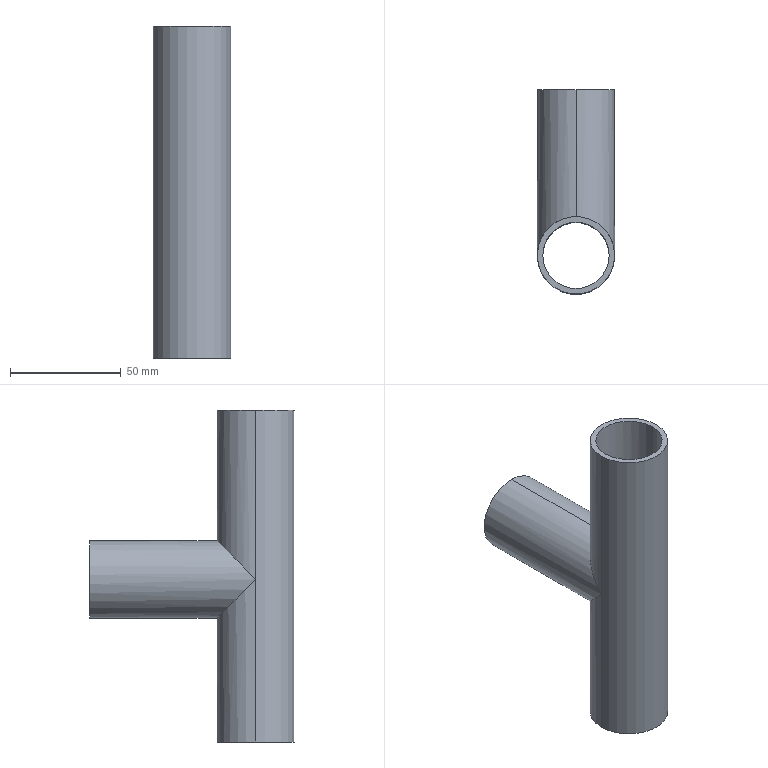Part | SolidWorks | features BaseBody 1 | 1 solid | 13 faces | box 35 x 92.5 x 150 mm | volume 52141 mm3 | cylinder 10 | plane 3 | commonest cylinder face diameters 30 x5 35 x5
STEP:
#1=CARTESIAN_POINT('',(-17.5,0.,150.));
#2=VERTEX_POINT('',#1);
#3=CARTESIAN_POINT('',(17.5,0.,150.));
#4=VERTEX_POINT('',#3);
#5=CARTESIAN_POINT('',(0.,0.,150.));
#6=DIRECTION('',(0.,0.,-1.));
#7=DIRECTION('',(-1.,0.,0.));
#8=AXIS2_PLACEMENT_3D('',#5,#6,#7);
#9=CIRCLE('',#8,17.5);
#10=EDGE_CURVE('',#2,#4,#9,.T.);
#11=ORIENTED_EDGE('',*,*,#10,.T.);
#12=CARTESIAN_POINT('',(17.5,0.,73.465));
#13=VERTEX_POINT('',#12);
#14=CARTESIAN_POINT('',(17.5,0.,150.));
#15=DIRECTION('',(0.,0.,-1.));
#16=VECTOR('',#15,1000.);
#17=LINE('',#14,#16);
#18=EDGE_CURVE('',#4,#13,#17,.T.);
#19=ORIENTED_EDGE('',*,*,#18,.T.);
#20=CARTESIAN_POINT('',(0.,17.5,90.965));
#21=VERTEX_POINT('',#20);
#22=CARTESIAN_POINT('',(17.5,0.,73.465));
#23=CARTESIAN_POINT('',(17.5,10.251,83.716));
#24=CARTESIAN_POINT('',(10.251,17.5,90.965));
#25=CARTESIAN_POINT('',(0.,17.5,90.965));
#26=(BOUNDED_CURVE()B_SPLINE_CURVE(3,(#22,#23,#24,#25),.UNSPECIFIED.,.F.,.T.)B_SPLINE_CURVE_WITH_KNOTS((4,4),(1.571,3.142),.UNSPECIFIED.)CURVE()GEOMETRIC_REPRESENTATION_ITEM()RATIONAL_B_SPLINE_CURVE((1.,0.8047,0.8047,1.))REPRESENTATION_ITEM(''));
#27=EDGE_CURVE('',#13,#21,#26,.T.);
#28=ORIENTED_EDGE('',*,*,#27,.T.);
#29=CARTESIAN_POINT('',(-17.5,0.,73.465));
#30=VERTEX_POINT('',#29);
#31=CARTESIAN_POINT('',(0.,17.5,90.965));
#32=CARTESIAN_POINT('',(-10.251,17.5,90.965));
#33=CARTESIAN_POINT('',(-17.5,10.251,83.716));
#34=CARTESIAN_POINT('',(-17.5,0.,73.465));
#35=(BOUNDED_CURVE()B_SPLINE_CURVE(3,(#31,#32,#33,#34),.UNSPECIFIED.,.F.,.F.)B_SPLINE_CURVE_WITH_KNOTS((4,4),(3.142,4.712),.UNSPECIFIED.)CURVE()GEOMETRIC_REPRESENTATION_ITEM()RATIONAL_B_SPLINE_CURVE((1.,0.8047,0.8047,1.))REPRESENTATION_ITEM(''));
#36=EDGE_CURVE('',#21,#30,#35,.T.);
#37=ORIENTED_EDGE('',*,*,#36,.T.);
#38=CARTESIAN_POINT('',(-17.5,0.,150.));
#39=DIRECTION('',(0.,0.,-1.));
#40=VECTOR('',#39,1000.);
#41=LINE('',#38,#40);
#42=EDGE_CURVE('',#2,#30,#41,.T.);
#43=ORIENTED_EDGE('',*,*,#42,.F.);
#44=EDGE_LOOP('',(#11,#19,#28,#37,#43));
#45=FACE_OUTER_BOUND('',#44,.T.);
#46=CARTESIAN_POINT('',(0.,0.,150.));
#47=DIRECTION('',(0.,0.,-1.));
#48=DIRECTION('',(-1.,0.,0.));
#49=AXIS2_PLACEMENT_3D('',#46,#47,#48);
#50=CYLINDRICAL_SURFACE('',#49,17.5);
#51=ADVANCED_FACE('',(#45),#50,.T.);
#52=CARTESIAN_POINT('',(0.,17.5,55.965));
#53=VERTEX_POINT('',#52);
#54=CARTESIAN_POINT('',(0.,17.5,55.965));
#55=CARTESIAN_POINT('',(10.251,17.5,55.965));
#56=CARTESIAN_POINT('',(17.5,10.251,63.213));
#57=CARTESIAN_POINT('',(17.5,0.,73.465));
#58=(BOUNDED_CURVE()B_SPLINE_CURVE(3,(#54,#55,#56,#57),.UNSPECIFIED.,.F.,.T.)B_SPLINE_CURVE_WITH_KNOTS((4,4),(3.142,4.712),.UNSPECIFIED.)CURVE()GEOMETRIC_REPRESENTATION_ITEM()RATIONAL_B_SPLINE_CURVE((1.,0.8047,0.8047,1.))REPRESENTATION_ITEM(''));
#59=EDGE_CURVE('',#53,#13,#58,.T.);
#60=ORIENTED_EDGE('',*,*,#59,.T.);
#61=CARTESIAN_POINT('',(17.5,0.,0.));
#62=VERTEX_POINT('',#61);
#63=CARTESIAN_POINT('',(17.5,0.,150.));
#64=DIRECTION('',(0.,0.,-1.));
#65=VECTOR('',#64,1000.);
#66=LINE('',#63,#65);
#67=EDGE_CURVE('',#13,#62,#66,.T.);
#68=ORIENTED_EDGE('',*,*,#67,.T.);
#69=CARTESIAN_POINT('',(-17.5,0.,0.));
#70=VERTEX_POINT('',#69);
#71=CARTESIAN_POINT('',(0.,0.,0.));
#72=DIRECTION('',(0.,0.,1.));
#73=DIRECTION('',(-1.,0.,0.));
#74=AXIS2_PLACEMENT_3D('',#71,#72,#73);
#75=CIRCLE('',#74,17.5);
#76=EDGE_CURVE('',#62,#70,#75,.T.);
#77=ORIENTED_EDGE('',*,*,#76,.T.);
#78=CARTESIAN_POINT('',(-17.5,0.,150.));
#79=DIRECTION('',(0.,0.,-1.));
#80=VECTOR('',#79,1000.);
#81=LINE('',#78,#80);
#82=EDGE_CURVE('',#30,#70,#81,.T.);
#83=ORIENTED_EDGE('',*,*,#82,.F.);
#84=CARTESIAN_POINT('',(-17.5,0.,73.465));
#85=CARTESIAN_POINT('',(-17.5,10.251,63.213));
#86=CARTESIAN_POINT('',(-10.251,17.5,55.965));
#87=CARTESIAN_POINT('',(0.,17.5,55.965));
#88=(BOUNDED_CURVE()B_SPLINE_CURVE(3,(#84,#85,#86,#87),.UNSPECIFIED.,.F.,.F.)B_SPLINE_CURVE_WITH_KNOTS((4,4),(1.571,3.142),.UNSPECIFIED.)CURVE()GEOMETRIC_REPRESENTATION_ITEM()RATIONAL_B_SPLINE_CURVE((1.,0.8047,0.8047,1.))REPRESENTATION_ITEM(''));
#89=EDGE_CURVE('',#30,#53,#88,.T.);
#90=ORIENTED_EDGE('',*,*,#89,.T.);
#91=EDGE_LOOP('',(#60,#68,#77,#83,#90));
#92=FACE_OUTER_BOUND('',#91,.T.);
#93=CARTESIAN_POINT('',(0.,0.,150.));
#94=DIRECTION('',(0.,0.,-1.));
#95=DIRECTION('',(-1.,0.,0.));
#96=AXIS2_PLACEMENT_3D('',#93,#94,#95);
#97=CYLINDRICAL_SURFACE('',#96,17.5);
#98=ADVANCED_FACE('',(#92),#97,.T.);
#99=CARTESIAN_POINT('',(0.,75.,55.965));
#100=VERTEX_POINT('',#99);
#101=CARTESIAN_POINT('',(0.,75.,90.965));
#102=VERTEX_POINT('',#101);
#103=CARTESIAN_POINT('',(0.,75.,73.465));
#104=DIRECTION('',(0.,-1.,0.));
#105=DIRECTION('',(0.,0.,-1.));
#106=AXIS2_PLACEMENT_3D('',#103,#104,#105);
#107=CIRCLE('',#106,17.5);
#108=EDGE_CURVE('',#100,#102,#107,.T.);
#109=ORIENTED_EDGE('',*,*,#108,.T.);
#110=CARTESIAN_POINT('',(0.,75.,90.965));
#111=DIRECTION('',(0.,-1.,0.));
#112=VECTOR('',#111,1000.);
#113=LINE('',#110,#112);
#114=EDGE_CURVE('',#102,#21,#113,.T.);
#115=ORIENTED_EDGE('',*,*,#114,.T.);
#116=ORIENTED_EDGE('',*,*,#27,.F.);
#117=ORIENTED_EDGE('',*,*,#59,.F.);
#118=CARTESIAN_POINT('',(0.,75.,55.965));
#119=DIRECTION('',(0.,-1.,0.));
#120=VECTOR('',#119,1000.);
#121=LINE('',#118,#120);
#122=EDGE_CURVE('',#100,#53,#121,.T.);
#123=ORIENTED_EDGE('',*,*,#122,.F.);
#124=EDGE_LOOP('',(#109,#115,#116,#117,#123));
#125=FACE_OUTER_BOUND('',#124,.T.);
#126=CARTESIAN_POINT('',(0.,75.,73.465));
#127=DIRECTION('',(0.,-1.,0.));
#128=DIRECTION('',(0.,0.,-1.));
#129=AXIS2_PLACEMENT_3D('',#126,#127,#128);
#130=CYLINDRICAL_SURFACE('',#129,17.5);
#131=ADVANCED_FACE('',(#125),#130,.T.);
#132=CARTESIAN_POINT('',(15.,0.,150.));
#133=VERTEX_POINT('',#132);
#134=CARTESIAN_POINT('',(-15.,0.,150.));
#135=VERTEX_POINT('',#134);
#136=CARTESIAN_POINT('',(0.,0.,150.));
#137=DIRECTION('',(0.,0.,-1.));
#138=DIRECTION('',(-1.,0.,0.));
#139=AXIS2_PLACEMENT_3D('',#136,#137,#138);
#140=CIRCLE('',#139,15.);
#141=EDGE_CURVE('',#133,#135,#140,.T.);
#142=ORIENTED_EDGE('',*,*,#141,.F.);
#143=CARTESIAN_POINT('',(15.,0.,73.465));
#144=VERTEX_POINT('',#143);
#145=CARTESIAN_POINT('',(15.,0.,150.));
#146=DIRECTION('',(0.,0.,-1.));
#147=VECTOR('',#146,1000.);
#148=LINE('',#145,#147);
#149=EDGE_CURVE('',#133,#144,#148,.T.);
#150=ORIENTED_EDGE('',*,*,#149,.T.);
#151=CARTESIAN_POINT('',(15.,0.,0.));
#152=VERTEX_POINT('',#151);
#153=CARTESIAN_POINT('',(15.,0.,150.));
#154=DIRECTION('',(0.,0.,-1.));
#155=VECTOR('',#154,1000.);
#156=LINE('',#153,#155);
#157=EDGE_CURVE('',#144,#152,#156,.T.);
#158=ORIENTED_EDGE('',*,*,#157,.T.);
#159=CARTESIAN_POINT('',(-15.,0.,0.));
#160=VERTEX_POINT('',#159);
#161=CARTESIAN_POINT('',(0.,0.,0.));
#162=DIRECTION('',(0.,0.,-1.));
#163=DIRECTION('',(-1.,0.,0.));
#164=AXIS2_PLACEMENT_3D('',#161,#162,#163);
#165=CIRCLE('',#164,15.);
#166=EDGE_CURVE('',#152,#160,#165,.T.);
#167=ORIENTED_EDGE('',*,*,#166,.T.);
#168=CARTESIAN_POINT('',(-15.,0.,73.465));
#169=VERTEX_POINT('',#168);
#170=CARTESIAN_POINT('',(-15.,0.,150.));
#171=DIRECTION('',(0.,0.,-1.));
#172=VECTOR('',#171,1000.);
#173=LINE('',#170,#172);
#174=EDGE_CURVE('',#169,#160,#173,.T.);
#175=ORIENTED_EDGE('',*,*,#174,.F.);
#176=CARTESIAN_POINT('',(-15.,0.,150.));
#177=DIRECTION('',(0.,0.,-1.));
#178=VECTOR('',#177,1000.);
#179=LINE('',#176,#178);
#180=EDGE_CURVE('',#135,#169,#179,.T.);
#181=ORIENTED_EDGE('',*,*,#180,.F.);
#182=EDGE_LOOP('',(#142,#150,#158,#167,#175,#181));
#183=FACE_OUTER_BOUND('',#182,.T.);
#184=CARTESIAN_POINT('',(0.,0.,150.));
#185=DIRECTION('',(0.,0.,-1.));
#186=DIRECTION('',(-1.,0.,0.));
#187=AXIS2_PLACEMENT_3D('',#184,#185,#186);
#188=CYLINDRICAL_SURFACE('',#187,15.);
#189=ADVANCED_FACE('',(#183),#188,.F.);
#190=ORIENTED_EDGE('',*,*,#149,.F.);
#191=CARTESIAN_POINT('',(0.,0.,150.));
#192=DIRECTION('',(0.,0.,-1.));
#193=DIRECTION('',(-1.,0.,0.));
#194=AXIS2_PLACEMENT_3D('',#191,#192,#193);
#195=CIRCLE('',#194,15.);
#196=EDGE_CURVE('',#135,#133,#195,.T.);
#197=ORIENTED_EDGE('',*,*,#196,.F.);
#198=ORIENTED_EDGE('',*,*,#180,.T.);
#199=CARTESIAN_POINT('',(0.,15.,88.465));
#200=VERTEX_POINT('',#199);
#201=CARTESIAN_POINT('',(0.,15.,88.465));
#202=CARTESIAN_POINT('',(-8.787,15.,88.465));
#203=CARTESIAN_POINT('',(-15.,8.787,82.251));
#204=CARTESIAN_POINT('',(-15.,0.,73.465));
#205=(BOUNDED_CURVE()B_SPLINE_CURVE(3,(#201,#202,#203,#204),.UNSPECIFIED.,.F.,.F.)B_SPLINE_CURVE_WITH_KNOTS((4,4),(0.,1.571),.UNSPECIFIED.)CURVE()GEOMETRIC_REPRESENTATION_ITEM()RATIONAL_B_SPLINE_CURVE((1.,0.8047,0.8047,1.))REPRESENTATION_ITEM(''));
#206=EDGE_CURVE('',#200,#169,#205,.T.);
#207=ORIENTED_EDGE('',*,*,#206,.F.);
#208=CARTESIAN_POINT('',(15.,0.,73.465));
#209=CARTESIAN_POINT('',(15.,8.787,82.251));
#210=CARTESIAN_POINT('',(8.787,15.,88.465));
#211=CARTESIAN_POINT('',(0.,15.,88.465));
#212=(BOUNDED_CURVE()B_SPLINE_CURVE(3,(#208,#209,#210,#211),.UNSPECIFIED.,.F.,.F.)B_SPLINE_CURVE_WITH_KNOTS((4,4),(4.712,6.283),.UNSPECIFIED.)CURVE()GEOMETRIC_REPRESENTATION_ITEM()RATIONAL_B_SPLINE_CURVE((1.,0.8047,0.8047,1.))REPRESENTATION_ITEM(''));
#213=EDGE_CURVE('',#144,#200,#212,.T.);
#214=ORIENTED_EDGE('',*,*,#213,.F.);
#215=EDGE_LOOP('',(#190,#197,#198,#207,#214));
#216=FACE_OUTER_BOUND('',#215,.T.);
#217=CARTESIAN_POINT('',(0.,0.,150.));
#218=DIRECTION('',(0.,0.,-1.));
#219=DIRECTION('',(-1.,0.,0.));
#220=AXIS2_PLACEMENT_3D('',#217,#218,#219);
#221=CYLINDRICAL_SURFACE('',#220,15.);
#222=ADVANCED_FACE('',(#216),#221,.F.);
#223=CARTESIAN_POINT('',(0.,15.,58.465));
#224=VERTEX_POINT('',#223);
#225=CARTESIAN_POINT('',(-15.,0.,73.465));
#226=CARTESIAN_POINT('',(-15.,8.787,64.678));
#227=CARTESIAN_POINT('',(-8.787,15.,58.465));
#228=CARTESIAN_POINT('',(0.,15.,58.465));
#229=(BOUNDED_CURVE()B_SPLINE_CURVE(3,(#225,#226,#227,#228),.UNSPECIFIED.,.F.,.F.)B_SPLINE_CURVE_WITH_KNOTS((4,4),(4.712,6.283),.UNSPECIFIED.)CURVE()GEOMETRIC_REPRESENTATION_ITEM()RATIONAL_B_SPLINE_CURVE((1.,0.8047,0.8047,1.))REPRESENTATION_ITEM(''));
#230=EDGE_CURVE('',#169,#224,#229,.T.);
#231=ORIENTED_EDGE('',*,*,#230,.T.);
#232=CARTESIAN_POINT('',(0.,75.,58.465));
#233=VERTEX_POINT('',#232);
#234=CARTESIAN_POINT('',(0.,0.,58.465));
#235=DIRECTION('',(0.,1.,0.));
#236=VECTOR('',#235,1000.);
#237=LINE('',#234,#236);
#238=EDGE_CURVE('',#224,#233,#237,.T.);
#239=ORIENTED_EDGE('',*,*,#238,.T.);
#240=CARTESIAN_POINT('',(0.,75.,88.465));
#241=VERTEX_POINT('',#240);
#242=CARTESIAN_POINT('',(0.,75.,73.465));
#243=DIRECTION('',(0.,-1.,0.));
#244=DIRECTION('',(0.,0.,1.));
#245=AXIS2_PLACEMENT_3D('',#242,#243,#244);
#246=CIRCLE('',#245,15.);
#247=EDGE_CURVE('',#241,#233,#246,.T.);
#248=ORIENTED_EDGE('',*,*,#247,.F.);
#249=CARTESIAN_POINT('',(0.,0.,88.465));
#250=DIRECTION('',(0.,1.,0.));
#251=VECTOR('',#250,1000.);
#252=LINE('',#249,#251);
#253=EDGE_CURVE('',#200,#241,#252,.T.);
#254=ORIENTED_EDGE('',*,*,#253,.F.);
#255=ORIENTED_EDGE('',*,*,#206,.T.);
#256=EDGE_LOOP('',(#231,#239,#248,#254,#255));
#257=FACE_OUTER_BOUND('',#256,.T.);
#258=CARTESIAN_POINT('',(0.,0.,73.465));
#259=DIRECTION('',(0.,1.,0.));
#260=DIRECTION('',(0.,0.,1.));
#261=AXIS2_PLACEMENT_3D('',#258,#259,#260);
#262=CYLINDRICAL_SURFACE('',#261,15.);
#263=ADVANCED_FACE('',(#257),#262,.F.);
#264=ORIENTED_EDGE('',*,*,#18,.F.);
#265=CARTESIAN_POINT('',(0.,0.,150.));
#266=DIRECTION('',(0.,0.,-1.));
#267=DIRECTION('',(-1.,0.,0.));
#268=AXIS2_PLACEMENT_3D('',#265,#266,#267);
#269=CIRCLE('',#268,17.5);
#270=EDGE_CURVE('',#4,#2,#269,.T.);
#271=ORIENTED_EDGE('',*,*,#270,.T.);
#272=ORIENTED_EDGE('',*,*,#42,.T.);
#273=ORIENTED_EDGE('',*,*,#82,.T.);
#274=CARTESIAN_POINT('',(0.,0.,0.));
#275=DIRECTION('',(0.,0.,1.));
#276=DIRECTION('',(-1.,0.,0.));
#277=AXIS2_PLACEMENT_3D('',#274,#275,#276);
#278=CIRCLE('',#277,17.5);
#279=EDGE_CURVE('',#70,#62,#278,.T.);
#280=ORIENTED_EDGE('',*,*,#279,.T.);
#281=ORIENTED_EDGE('',*,*,#67,.F.);
#282=EDGE_LOOP('',(#264,#271,#272,#273,#280,#281));
#283=FACE_OUTER_BOUND('',#282,.T.);
#284=CARTESIAN_POINT('',(0.,0.,150.));
#285=DIRECTION('',(0.,0.,-1.));
#286=DIRECTION('',(-1.,0.,0.));
#287=AXIS2_PLACEMENT_3D('',#284,#285,#286);
#288=CYLINDRICAL_SURFACE('',#287,17.5);
#289=ADVANCED_FACE('',(#283),#288,.T.);
#290=CARTESIAN_POINT('',(0.,0.,0.));
#291=DIRECTION('',(0.,0.,-1.));
#292=DIRECTION('',(-1.,0.,0.));
#293=AXIS2_PLACEMENT_3D('',#290,#291,#292);
#294=CIRCLE('',#293,15.);
#295=EDGE_CURVE('',#160,#152,#294,.T.);
#296=ORIENTED_EDGE('',*,*,#295,.F.);
#297=ORIENTED_EDGE('',*,*,#166,.F.);
#298=EDGE_LOOP('',(#296,#297));
#299=FACE_BOUND('',#298,.T.);
#300=ORIENTED_EDGE('',*,*,#279,.F.);
#301=ORIENTED_EDGE('',*,*,#76,.F.);
#302=EDGE_LOOP('',(#300,#301));
#303=FACE_OUTER_BOUND('',#302,.T.);
#304=CARTESIAN_POINT('',(0.,0.,0.));
#305=DIRECTION('',(0.,0.,1.));
#306=DIRECTION('',(1.,0.,0.));
#307=AXIS2_PLACEMENT_3D('',#304,#305,#306);
#308=PLANE('',#307);
#309=ADVANCED_FACE('',(#299,#303),#308,.F.);
#310=ORIENTED_EDGE('',*,*,#196,.T.);
#311=ORIENTED_EDGE('',*,*,#141,.T.);
#312=EDGE_LOOP('',(#310,#311));
#313=FACE_BOUND('',#312,.T.);
#314=ORIENTED_EDGE('',*,*,#10,.F.);
#315=ORIENTED_EDGE('',*,*,#270,.F.);
#316=EDGE_LOOP('',(#314,#315));
#317=FACE_OUTER_BOUND('',#316,.T.);
#318=CARTESIAN_POINT('',(0.,0.,150.));
#319=DIRECTION('',(0.,0.,1.));
#320=DIRECTION('',(1.,0.,0.));
#321=AXIS2_PLACEMENT_3D('',#318,#319,#320);
#322=PLANE('',#321);
#323=ADVANCED_FACE('',(#313,#317),#322,.T.);
#324=ORIENTED_EDGE('',*,*,#114,.F.);
#325=CARTESIAN_POINT('',(0.,75.,73.465));
#326=DIRECTION('',(0.,-1.,0.));
#327=DIRECTION('',(0.,0.,-1.));
#328=AXIS2_PLACEMENT_3D('',#325,#326,#327);
#329=CIRCLE('',#328,17.5);
#330=EDGE_CURVE('',#102,#100,#329,.T.);
#331=ORIENTED_EDGE('',*,*,#330,.T.);
#332=ORIENTED_EDGE('',*,*,#122,.T.);
#333=ORIENTED_EDGE('',*,*,#89,.F.);
#334=ORIENTED_EDGE('',*,*,#36,.F.);
#335=EDGE_LOOP('',(#324,#331,#332,#333,#334));
#336=FACE_OUTER_BOUND('',#335,.T.);
#337=CARTESIAN_POINT('',(0.,75.,73.465));
#338=DIRECTION('',(0.,-1.,0.));
#339=DIRECTION('',(0.,0.,-1.));
#340=AXIS2_PLACEMENT_3D('',#337,#338,#339);
#341=CYLINDRICAL_SURFACE('',#340,17.5);
#342=ADVANCED_FACE('',(#336),#341,.T.);
#343=ORIENTED_EDGE('',*,*,#157,.F.);
#344=CARTESIAN_POINT('',(0.,15.,58.465));
#345=CARTESIAN_POINT('',(8.787,15.,58.465));
#346=CARTESIAN_POINT('',(15.,8.787,64.678));
#347=CARTESIAN_POINT('',(15.,0.,73.465));
#348=(BOUNDED_CURVE()B_SPLINE_CURVE(3,(#344,#345,#346,#347),.UNSPECIFIED.,.F.,.F.)B_SPLINE_CURVE_WITH_KNOTS((4,4),(0.,1.571),.UNSPECIFIED.)CURVE()GEOMETRIC_REPRESENTATION_ITEM()RATIONAL_B_SPLINE_CURVE((1.,0.8047,0.8047,1.))REPRESENTATION_ITEM(''));
#349=EDGE_CURVE('',#224,#144,#348,.T.);
#350=ORIENTED_EDGE('',*,*,#349,.F.);
#351=ORIENTED_EDGE('',*,*,#230,.F.);
#352=ORIENTED_EDGE('',*,*,#174,.T.);
#353=ORIENTED_EDGE('',*,*,#295,.T.);
#354=EDGE_LOOP('',(#343,#350,#351,#352,#353));
#355=FACE_OUTER_BOUND('',#354,.T.);
#356=CARTESIAN_POINT('',(0.,0.,150.));
#357=DIRECTION('',(0.,0.,-1.));
#358=DIRECTION('',(-1.,0.,0.));
#359=AXIS2_PLACEMENT_3D('',#356,#357,#358);
#360=CYLINDRICAL_SURFACE('',#359,15.);
#361=ADVANCED_FACE('',(#355),#360,.F.);
#362=ORIENTED_EDGE('',*,*,#108,.F.);
#363=ORIENTED_EDGE('',*,*,#330,.F.);
#364=EDGE_LOOP('',(#362,#363));
#365=FACE_OUTER_BOUND('',#364,.T.);
#366=ORIENTED_EDGE('',*,*,#247,.T.);
#367=CARTESIAN_POINT('',(0.,75.,73.465));
#368=DIRECTION('',(0.,-1.,0.));
#369=DIRECTION('',(0.,0.,1.));
#370=AXIS2_PLACEMENT_3D('',#367,#368,#369);
#371=CIRCLE('',#370,15.);
#372=EDGE_CURVE('',#233,#241,#371,.T.);
#373=ORIENTED_EDGE('',*,*,#372,.T.);
#374=EDGE_LOOP('',(#366,#373));
#375=FACE_BOUND('',#374,.T.);
#376=CARTESIAN_POINT('',(0.,75.,73.465));
#377=DIRECTION('',(0.,1.,0.));
#378=DIRECTION('',(0.,0.,1.));
#379=AXIS2_PLACEMENT_3D('',#376,#377,#378);
#380=PLANE('',#379);
#381=ADVANCED_FACE('',(#365,#375),#380,.T.);
#382=ORIENTED_EDGE('',*,*,#238,.F.);
#383=ORIENTED_EDGE('',*,*,#349,.T.);
#384=ORIENTED_EDGE('',*,*,#213,.T.);
#385=ORIENTED_EDGE('',*,*,#253,.T.);
#386=ORIENTED_EDGE('',*,*,#372,.F.);
#387=EDGE_LOOP('',(#382,#383,#384,#385,#386));
#388=FACE_OUTER_BOUND('',#387,.T.);
#389=CARTESIAN_POINT('',(0.,0.,73.465));
#390=DIRECTION('',(0.,1.,0.));
#391=DIRECTION('',(0.,0.,1.));
#392=AXIS2_PLACEMENT_3D('',#389,#390,#391);
#393=CYLINDRICAL_SURFACE('',#392,15.);
#394=ADVANCED_FACE('',(#388),#393,.F.);
#395=CLOSED_SHELL('',(#51,#98,#131,#189,#222,#263,#289,#309,#323,#342,#361,#381,#394));
#396=MANIFOLD_SOLID_BREP('',#395);
#397=CARTESIAN_POINT('',(0.,0.,0.));
#398=DIRECTION('',(0.,0.,1.));
#399=DIRECTION('',(1.,0.,0.));
#400=AXIS2_PLACEMENT_3D('',#397,#398,#399);
#401=(LENGTH_UNIT()NAMED_UNIT(*)SI_UNIT(.MILLI.,.METRE.));
#402=UNCERTAINTY_MEASURE_WITH_UNIT(LENGTH_MEASURE(0.00001),#401,'','');
#403=(NAMED_UNIT(*)PLANE_ANGLE_UNIT()SI_UNIT($,.RADIAN.));
#404=(NAMED_UNIT(*)SI_UNIT($,.STERADIAN.)SOLID_ANGLE_UNIT());
#405=(GEOMETRIC_REPRESENTATION_CONTEXT(3)GLOBAL_UNCERTAINTY_ASSIGNED_CONTEXT((#402))GLOBAL_UNIT_ASSIGNED_CONTEXT((#401,#403,#404))REPRESENTATION_CONTEXT('',''));
#406=ADVANCED_BREP_SHAPE_REPRESENTATION('',(#396,#400),#405);